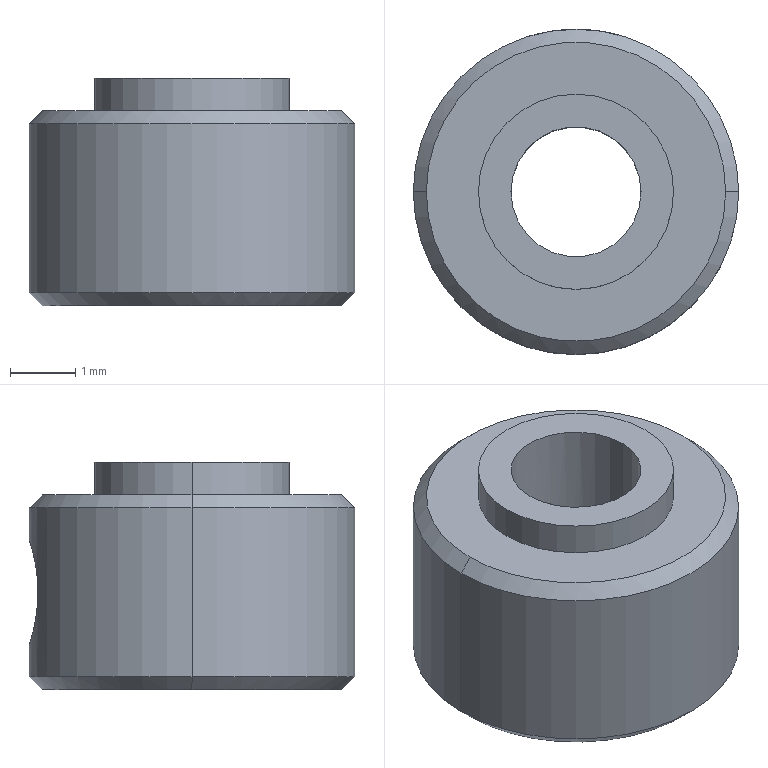Part | SolidWorks | features Chamfer 1, Extrusion 1, HoleWzd 1, ICE 1 | 1 solid | 15 faces | box 5 x 5 x 3.5 mm | volume 47.704 mm3 | cylinder 8 | cone 4 | plane 3 | commonest cylinder face diameters 1.6 x2 2 x2 3 x2 5 x2
STEP:
#1=CARTESIAN_POINT('',(2.3,0.,1.5));
#2=VERTEX_POINT('',#1);
#3=CARTESIAN_POINT('',(-2.3,0.,1.5));
#4=VERTEX_POINT('',#3);
#5=CARTESIAN_POINT('',(0.,0.,1.5));
#6=DIRECTION('',(0.,0.,1.));
#7=DIRECTION('',(1.,0.,0.));
#8=AXIS2_PLACEMENT_3D('',#5,#6,#7);
#9=CIRCLE('',#8,2.3);
#10=EDGE_CURVE('',#2,#4,#9,.T.);
#11=ORIENTED_EDGE('',*,*,#10,.F.);
#12=CARTESIAN_POINT('',(2.5,0.,1.3));
#13=VERTEX_POINT('',#12);
#14=CARTESIAN_POINT('',(2.3,0.,1.5));
#15=DIRECTION('',(0.7071,0.,-0.7071));
#16=VECTOR('',#15,1000.);
#17=LINE('',#14,#16);
#18=EDGE_CURVE('',#2,#13,#17,.T.);
#19=ORIENTED_EDGE('',*,*,#18,.T.);
#20=CARTESIAN_POINT('',(-2.5,0.,1.3));
#21=VERTEX_POINT('',#20);
#22=CARTESIAN_POINT('',(0.,0.,1.3));
#23=DIRECTION('',(0.,0.,-1.));
#24=DIRECTION('',(1.,0.,0.));
#25=AXIS2_PLACEMENT_3D('',#22,#23,#24);
#26=CIRCLE('',#25,2.5);
#27=EDGE_CURVE('',#21,#13,#26,.T.);
#28=ORIENTED_EDGE('',*,*,#27,.F.);
#29=CARTESIAN_POINT('',(-2.3,0.,1.5));
#30=DIRECTION('',(-0.7071,0.,-0.7071));
#31=VECTOR('',#30,1000.);
#32=LINE('',#29,#31);
#33=EDGE_CURVE('',#4,#21,#32,.T.);
#34=ORIENTED_EDGE('',*,*,#33,.F.);
#35=EDGE_LOOP('',(#11,#19,#28,#34));
#36=FACE_OUTER_BOUND('',#35,.T.);
#37=CARTESIAN_POINT('',(0.,0.,1.5));
#38=DIRECTION('',(0.,0.,-1.));
#39=DIRECTION('',(-1.,0.,0.));
#40=AXIS2_PLACEMENT_3D('',#37,#38,#39);
#41=CONICAL_SURFACE('',#40,2.3,0.7854);
#42=ADVANCED_FACE('',(#36),#41,.T.);
#43=CARTESIAN_POINT('',(-2.3,0.,-1.5));
#44=VERTEX_POINT('',#43);
#45=CARTESIAN_POINT('',(2.3,0.,-1.5));
#46=VERTEX_POINT('',#45);
#47=CARTESIAN_POINT('',(0.,0.,-1.5));
#48=DIRECTION('',(0.,0.,-1.));
#49=DIRECTION('',(1.,0.,0.));
#50=AXIS2_PLACEMENT_3D('',#47,#48,#49);
#51=CIRCLE('',#50,2.3);
#52=EDGE_CURVE('',#44,#46,#51,.T.);
#53=ORIENTED_EDGE('',*,*,#52,.F.);
#54=CARTESIAN_POINT('',(-2.5,0.,-1.3));
#55=VERTEX_POINT('',#54);
#56=CARTESIAN_POINT('',(-2.5,0.,-1.3));
#57=DIRECTION('',(-0.7071,0.,0.7071));
#58=VECTOR('',#57,1000.);
#59=LINE('',#56,#58);
#60=EDGE_CURVE('',#44,#55,#59,.T.);
#61=ORIENTED_EDGE('',*,*,#60,.T.);
#62=CARTESIAN_POINT('',(2.5,0.,-1.3));
#63=VERTEX_POINT('',#62);
#64=CARTESIAN_POINT('',(0.,0.,-1.3));
#65=DIRECTION('',(0.,0.,1.));
#66=DIRECTION('',(1.,0.,0.));
#67=AXIS2_PLACEMENT_3D('',#64,#65,#66);
#68=CIRCLE('',#67,2.5);
#69=EDGE_CURVE('',#63,#55,#68,.T.);
#70=ORIENTED_EDGE('',*,*,#69,.F.);
#71=CARTESIAN_POINT('',(2.5,0.,-1.3));
#72=DIRECTION('',(0.7071,0.,0.7071));
#73=VECTOR('',#72,1000.);
#74=LINE('',#71,#73);
#75=EDGE_CURVE('',#46,#63,#74,.T.);
#76=ORIENTED_EDGE('',*,*,#75,.F.);
#77=EDGE_LOOP('',(#53,#61,#70,#76));
#78=FACE_OUTER_BOUND('',#77,.T.);
#79=CARTESIAN_POINT('',(0.,0.,-1.3));
#80=DIRECTION('',(0.,0.,1.));
#81=DIRECTION('',(1.,0.,0.));
#82=AXIS2_PLACEMENT_3D('',#79,#80,#81);
#83=CONICAL_SURFACE('',#82,2.5,0.7854);
#84=ADVANCED_FACE('',(#78),#83,.T.);
#85=CARTESIAN_POINT('',(0.,2.5,0.8));
#86=VERTEX_POINT('',#85);
#87=CARTESIAN_POINT('',(0.,2.5,-0.8));
#88=VERTEX_POINT('',#87);
#89=CARTESIAN_POINT('',(0.,2.5,0.8));
#90=CARTESIAN_POINT('',(-0.1049,2.5,0.8));
#91=CARTESIAN_POINT('',(-0.2107,2.493,0.7788));
#92=CARTESIAN_POINT('',(-0.4037,2.469,0.6985));
#93=CARTESIAN_POINT('',(-0.4919,2.452,0.6395));
#94=CARTESIAN_POINT('',(-0.6396,2.418,0.4918));
#95=CARTESIAN_POINT('',(-0.6982,2.401,0.4046));
#96=CARTESIAN_POINT('',(-0.7791,2.376,0.2099));
#97=CARTESIAN_POINT('',(-0.8,2.369,0.1054));
#98=CARTESIAN_POINT('',(-0.8,2.369,-0.1055));
#99=CARTESIAN_POINT('',(-0.7787,2.376,-0.211));
#100=CARTESIAN_POINT('',(-0.6986,2.401,-0.4036));
#101=CARTESIAN_POINT('',(-0.6391,2.418,-0.4922));
#102=CARTESIAN_POINT('',(-0.4925,2.452,-0.6389));
#103=CARTESIAN_POINT('',(-0.4043,2.469,-0.6982));
#104=CARTESIAN_POINT('',(-0.2111,2.493,-0.7787));
#105=CARTESIAN_POINT('',(-0.1064,2.5,-0.8));
#106=CARTESIAN_POINT('',(0.,2.5,-0.8));
#107=B_SPLINE_CURVE_WITH_KNOTS('',3,(#89,#90,#91,#92,#93,#94,#95,#96,#97,#98,#99,#100,#101,#102,#103,#104,#105,#106),.UNSPECIFIED.,.F.,.F.,(4,2,2,2,2,2,2,2,4),(0.002518,0.002832,0.003147,0.003462,0.003776,0.004091,0.004406,0.00472,0.005035),.UNSPECIFIED.);
#108=EDGE_CURVE('',#86,#88,#107,.T.);
#109=ORIENTED_EDGE('',*,*,#108,.F.);
#110=CARTESIAN_POINT('',(0.,1.,0.8));
#111=VERTEX_POINT('',#110);
#112=CARTESIAN_POINT('',(0.,0.,0.8));
#113=DIRECTION('',(0.,-1.,0.));
#114=VECTOR('',#113,1000.);
#115=LINE('',#112,#114);
#116=EDGE_CURVE('',#86,#111,#115,.T.);
#117=ORIENTED_EDGE('',*,*,#116,.T.);
#118=CARTESIAN_POINT('',(0.,1.,-0.8));
#119=VERTEX_POINT('',#118);
#120=CARTESIAN_POINT('',(0.,1.,0.8));
#121=CARTESIAN_POINT('',(-0.1101,1.,0.8));
#122=CARTESIAN_POINT('',(-0.2209,0.9807,0.7762));
#123=CARTESIAN_POINT('',(-0.4161,0.9151,0.6915));
#124=CARTESIAN_POINT('',(-0.5007,0.8698,0.6318));
#125=CARTESIAN_POINT('',(-0.6401,0.7729,0.49));
#126=CARTESIAN_POINT('',(-0.6961,0.7204,0.4071));
#127=CARTESIAN_POINT('',(-0.7755,0.6341,0.2211));
#128=CARTESIAN_POINT('',(-0.7999,0.6001,0.1121));
#129=CARTESIAN_POINT('',(-0.8001,0.5999,-0.1109));
#130=CARTESIAN_POINT('',(-0.7764,0.6331,-0.2186));
#131=CARTESIAN_POINT('',(-0.6962,0.7203,-0.4072));
#132=CARTESIAN_POINT('',(-0.641,0.7723,-0.489));
#133=CARTESIAN_POINT('',(-0.5007,0.8698,-0.6319));
#134=CARTESIAN_POINT('',(-0.4177,0.9144,-0.6906));
#135=CARTESIAN_POINT('',(-0.2225,0.9804,-0.7758));
#136=CARTESIAN_POINT('',(-0.1119,1.,-0.8));
#137=CARTESIAN_POINT('',(0.,1.,-0.8));
#138=B_SPLINE_CURVE_WITH_KNOTS('',3,(#120,#121,#122,#123,#124,#125,#126,#127,#128,#129,#130,#131,#132,#133,#134,#135,#136,#137),.UNSPECIFIED.,.F.,.F.,(4,2,2,2,2,2,2,2,4),(0.002649,0.002979,0.003309,0.003639,0.003969,0.004299,0.00463,0.00496,0.00529),.UNSPECIFIED.);
#139=EDGE_CURVE('',#111,#119,#138,.T.);
#140=ORIENTED_EDGE('',*,*,#139,.T.);
#141=CARTESIAN_POINT('',(0.,0.,-0.8));
#142=DIRECTION('',(0.,-1.,0.));
#143=VECTOR('',#142,1000.);
#144=LINE('',#141,#143);
#145=EDGE_CURVE('',#88,#119,#144,.T.);
#146=ORIENTED_EDGE('',*,*,#145,.F.);
#147=EDGE_LOOP('',(#109,#117,#140,#146));
#148=FACE_OUTER_BOUND('',#147,.T.);
#149=CARTESIAN_POINT('',(0.,0.,0.));
#150=DIRECTION('',(0.,-1.,0.));
#151=DIRECTION('',(0.,0.,-1.));
#152=AXIS2_PLACEMENT_3D('',#149,#150,#151);
#153=CYLINDRICAL_SURFACE('',#152,0.8);
#154=ADVANCED_FACE('',(#148),#153,.F.);
#155=CARTESIAN_POINT('',(1.5,0.,2.));
#156=VERTEX_POINT('',#155);
#157=CARTESIAN_POINT('',(-1.5,0.,2.));
#158=VERTEX_POINT('',#157);
#159=CARTESIAN_POINT('',(0.,0.,2.));
#160=DIRECTION('',(0.,0.,1.));
#161=DIRECTION('',(1.,0.,0.));
#162=AXIS2_PLACEMENT_3D('',#159,#160,#161);
#163=CIRCLE('',#162,1.5);
#164=EDGE_CURVE('',#156,#158,#163,.T.);
#165=ORIENTED_EDGE('',*,*,#164,.F.);
#166=CARTESIAN_POINT('',(1.5,0.,1.5));
#167=VERTEX_POINT('',#166);
#168=CARTESIAN_POINT('',(1.5,0.,2.));
#169=DIRECTION('',(0.,0.,-1.));
#170=VECTOR('',#169,1000.);
#171=LINE('',#168,#170);
#172=EDGE_CURVE('',#156,#167,#171,.T.);
#173=ORIENTED_EDGE('',*,*,#172,.T.);
#174=CARTESIAN_POINT('',(-1.5,0.,1.5));
#175=VERTEX_POINT('',#174);
#176=CARTESIAN_POINT('',(0.,0.,1.5));
#177=DIRECTION('',(0.,0.,1.));
#178=DIRECTION('',(1.,0.,0.));
#179=AXIS2_PLACEMENT_3D('',#176,#177,#178);
#180=CIRCLE('',#179,1.5);
#181=EDGE_CURVE('',#167,#175,#180,.T.);
#182=ORIENTED_EDGE('',*,*,#181,.T.);
#183=CARTESIAN_POINT('',(-1.5,0.,2.));
#184=DIRECTION('',(0.,0.,-1.));
#185=VECTOR('',#184,1000.);
#186=LINE('',#183,#185);
#187=EDGE_CURVE('',#158,#175,#186,.T.);
#188=ORIENTED_EDGE('',*,*,#187,.F.);
#189=EDGE_LOOP('',(#165,#173,#182,#188));
#190=FACE_OUTER_BOUND('',#189,.T.);
#191=CARTESIAN_POINT('',(0.,0.,2.));
#192=DIRECTION('',(0.,0.,-1.));
#193=DIRECTION('',(-1.,0.,0.));
#194=AXIS2_PLACEMENT_3D('',#191,#192,#193);
#195=CYLINDRICAL_SURFACE('',#194,1.5);
#196=ADVANCED_FACE('',(#190),#195,.T.);
#197=CARTESIAN_POINT('',(-1.,0.,2.));
#198=VERTEX_POINT('',#197);
#199=CARTESIAN_POINT('',(1.,0.,2.));
#200=VERTEX_POINT('',#199);
#201=CARTESIAN_POINT('',(0.,0.,2.));
#202=DIRECTION('',(0.,0.,1.));
#203=DIRECTION('',(1.,0.,0.));
#204=AXIS2_PLACEMENT_3D('',#201,#202,#203);
#205=CIRCLE('',#204,1.);
#206=EDGE_CURVE('',#198,#200,#205,.T.);
#207=ORIENTED_EDGE('',*,*,#206,.T.);
#208=CARTESIAN_POINT('',(1.,0.,-1.5));
#209=VERTEX_POINT('',#208);
#210=CARTESIAN_POINT('',(1.,0.,1.5));
#211=DIRECTION('',(0.,0.,-1.));
#212=VECTOR('',#211,1000.);
#213=LINE('',#210,#212);
#214=EDGE_CURVE('',#200,#209,#213,.T.);
#215=ORIENTED_EDGE('',*,*,#214,.T.);
#216=CARTESIAN_POINT('',(-1.,0.,-1.5));
#217=VERTEX_POINT('',#216);
#218=CARTESIAN_POINT('',(0.,0.,-1.5));
#219=DIRECTION('',(0.,0.,1.));
#220=DIRECTION('',(1.,0.,0.));
#221=AXIS2_PLACEMENT_3D('',#218,#219,#220);
#222=CIRCLE('',#221,1.);
#223=EDGE_CURVE('',#217,#209,#222,.T.);
#224=ORIENTED_EDGE('',*,*,#223,.F.);
#225=CARTESIAN_POINT('',(-1.,0.,1.5));
#226=DIRECTION('',(0.,0.,-1.));
#227=VECTOR('',#226,1000.);
#228=LINE('',#225,#227);
#229=EDGE_CURVE('',#198,#217,#228,.T.);
#230=ORIENTED_EDGE('',*,*,#229,.F.);
#231=EDGE_LOOP('',(#207,#215,#224,#230));
#232=FACE_OUTER_BOUND('',#231,.T.);
#233=CARTESIAN_POINT('',(0.,0.,1.5));
#234=DIRECTION('',(0.,0.,-1.));
#235=DIRECTION('',(-1.,0.,0.));
#236=AXIS2_PLACEMENT_3D('',#233,#234,#235);
#237=CYLINDRICAL_SURFACE('',#236,1.);
#238=ADVANCED_FACE('',(#232),#237,.F.);
#239=CARTESIAN_POINT('',(0.,2.5,-0.8));
#240=CARTESIAN_POINT('',(0.1065,2.5,-0.8));
#241=CARTESIAN_POINT('',(0.2109,2.493,-0.7788));
#242=CARTESIAN_POINT('',(0.4044,2.469,-0.6982));
#243=CARTESIAN_POINT('',(0.4927,2.452,-0.6388));
#244=CARTESIAN_POINT('',(0.6392,2.418,-0.4921));
#245=CARTESIAN_POINT('',(0.6986,2.401,-0.4035));
#246=CARTESIAN_POINT('',(0.7786,2.376,-0.2113));
#247=CARTESIAN_POINT('',(0.7999,2.369,-0.1055));
#248=CARTESIAN_POINT('',(0.8001,2.369,0.1048));
#249=CARTESIAN_POINT('',(0.7791,2.376,0.2099));
#250=CARTESIAN_POINT('',(0.6982,2.401,0.4045));
#251=CARTESIAN_POINT('',(0.6392,2.418,0.4922));
#252=CARTESIAN_POINT('',(0.4917,2.452,0.6396));
#253=CARTESIAN_POINT('',(0.4035,2.469,0.6986));
#254=CARTESIAN_POINT('',(0.2107,2.493,0.7788));
#255=CARTESIAN_POINT('',(0.1049,2.5,0.8));
#256=CARTESIAN_POINT('',(0.,2.5,0.8));
#257=B_SPLINE_CURVE_WITH_KNOTS('',3,(#239,#240,#241,#242,#243,#244,#245,#246,#247,#248,#249,#250,#251,#252,#253,#254,#255,#256),.UNSPECIFIED.,.F.,.F.,(4,2,2,2,2,2,2,2,4),(0.,0.0003147,0.0006295,0.0009442,0.001259,0.001574,0.001888,0.002203,0.002518),.UNSPECIFIED.);
#258=EDGE_CURVE('',#88,#86,#257,.T.);
#259=ORIENTED_EDGE('',*,*,#258,.T.);
#260=ORIENTED_EDGE('',*,*,#108,.T.);
#261=EDGE_LOOP('',(#259,#260));
#262=FACE_BOUND('',#261,.T.);
#263=ORIENTED_EDGE('',*,*,#27,.T.);
#264=CARTESIAN_POINT('',(2.5,0.,1.5));
#265=DIRECTION('',(0.,0.,-1.));
#266=VECTOR('',#265,1000.);
#267=LINE('',#264,#266);
#268=EDGE_CURVE('',#13,#63,#267,.T.);
#269=ORIENTED_EDGE('',*,*,#268,.T.);
#270=ORIENTED_EDGE('',*,*,#69,.T.);
#271=CARTESIAN_POINT('',(-2.5,0.,1.5));
#272=DIRECTION('',(0.,0.,-1.));
#273=VECTOR('',#272,1000.);
#274=LINE('',#271,#273);
#275=EDGE_CURVE('',#21,#55,#274,.T.);
#276=ORIENTED_EDGE('',*,*,#275,.F.);
#277=EDGE_LOOP('',(#263,#269,#270,#276));
#278=FACE_OUTER_BOUND('',#277,.T.);
#279=CARTESIAN_POINT('',(0.,0.,1.5));
#280=DIRECTION('',(0.,0.,-1.));
#281=DIRECTION('',(-1.,0.,0.));
#282=AXIS2_PLACEMENT_3D('',#279,#280,#281);
#283=CYLINDRICAL_SURFACE('',#282,2.5);
#284=ADVANCED_FACE('',(#262,#278),#283,.T.);
#285=CARTESIAN_POINT('',(0.,0.,1.5));
#286=DIRECTION('',(0.,0.,1.));
#287=DIRECTION('',(1.,0.,0.));
#288=AXIS2_PLACEMENT_3D('',#285,#286,#287);
#289=CIRCLE('',#288,2.3);
#290=EDGE_CURVE('',#4,#2,#289,.T.);
#291=ORIENTED_EDGE('',*,*,#290,.T.);
#292=ORIENTED_EDGE('',*,*,#10,.T.);
#293=EDGE_LOOP('',(#291,#292));
#294=FACE_OUTER_BOUND('',#293,.T.);
#295=CARTESIAN_POINT('',(0.,0.,1.5));
#296=DIRECTION('',(0.,0.,1.));
#297=DIRECTION('',(1.,0.,0.));
#298=AXIS2_PLACEMENT_3D('',#295,#296,#297);
#299=CIRCLE('',#298,1.5);
#300=EDGE_CURVE('',#175,#167,#299,.T.);
#301=ORIENTED_EDGE('',*,*,#300,.F.);
#302=ORIENTED_EDGE('',*,*,#181,.F.);
#303=EDGE_LOOP('',(#301,#302));
#304=FACE_BOUND('',#303,.T.);
#305=CARTESIAN_POINT('',(0.,0.,1.5));
#306=DIRECTION('',(0.,0.,1.));
#307=DIRECTION('',(1.,0.,0.));
#308=AXIS2_PLACEMENT_3D('',#305,#306,#307);
#309=PLANE('',#308);
#310=ADVANCED_FACE('',(#294,#304),#309,.T.);
#311=CARTESIAN_POINT('',(0.,0.,-1.5));
#312=DIRECTION('',(0.,0.,-1.));
#313=DIRECTION('',(1.,0.,0.));
#314=AXIS2_PLACEMENT_3D('',#311,#312,#313);
#315=CIRCLE('',#314,2.3);
#316=EDGE_CURVE('',#46,#44,#315,.T.);
#317=ORIENTED_EDGE('',*,*,#316,.T.);
#318=ORIENTED_EDGE('',*,*,#52,.T.);
#319=EDGE_LOOP('',(#317,#318));
#320=FACE_OUTER_BOUND('',#319,.T.);
#321=ORIENTED_EDGE('',*,*,#223,.T.);
#322=CARTESIAN_POINT('',(0.,0.,-1.5));
#323=DIRECTION('',(0.,0.,1.));
#324=DIRECTION('',(1.,0.,0.));
#325=AXIS2_PLACEMENT_3D('',#322,#323,#324);
#326=CIRCLE('',#325,1.);
#327=EDGE_CURVE('',#209,#217,#326,.T.);
#328=ORIENTED_EDGE('',*,*,#327,.T.);
#329=EDGE_LOOP('',(#321,#328));
#330=FACE_BOUND('',#329,.T.);
#331=CARTESIAN_POINT('',(0.,0.,-1.5));
#332=DIRECTION('',(0.,0.,1.));
#333=DIRECTION('',(1.,0.,0.));
#334=AXIS2_PLACEMENT_3D('',#331,#332,#333);
#335=PLANE('',#334);
#336=ADVANCED_FACE('',(#320,#330),#335,.F.);
#337=ORIENTED_EDGE('',*,*,#268,.F.);
#338=CARTESIAN_POINT('',(0.,0.,1.3));
#339=DIRECTION('',(0.,0.,-1.));
#340=DIRECTION('',(1.,0.,0.));
#341=AXIS2_PLACEMENT_3D('',#338,#339,#340);
#342=CIRCLE('',#341,2.5);
#343=EDGE_CURVE('',#13,#21,#342,.T.);
#344=ORIENTED_EDGE('',*,*,#343,.T.);
#345=ORIENTED_EDGE('',*,*,#275,.T.);
#346=CARTESIAN_POINT('',(0.,0.,-1.3));
#347=DIRECTION('',(0.,0.,1.));
#348=DIRECTION('',(1.,0.,0.));
#349=AXIS2_PLACEMENT_3D('',#346,#347,#348);
#350=CIRCLE('',#349,2.5);
#351=EDGE_CURVE('',#55,#63,#350,.T.);
#352=ORIENTED_EDGE('',*,*,#351,.T.);
#353=EDGE_LOOP('',(#337,#344,#345,#352));
#354=FACE_OUTER_BOUND('',#353,.T.);
#355=CARTESIAN_POINT('',(0.,0.,1.5));
#356=DIRECTION('',(0.,0.,-1.));
#357=DIRECTION('',(-1.,0.,0.));
#358=AXIS2_PLACEMENT_3D('',#355,#356,#357);
#359=CYLINDRICAL_SURFACE('',#358,2.5);
#360=ADVANCED_FACE('',(#354),#359,.T.);
#361=ORIENTED_EDGE('',*,*,#214,.F.);
#362=CARTESIAN_POINT('',(0.,0.,2.));
#363=DIRECTION('',(0.,0.,1.));
#364=DIRECTION('',(1.,0.,0.));
#365=AXIS2_PLACEMENT_3D('',#362,#363,#364);
#366=CIRCLE('',#365,1.);
#367=EDGE_CURVE('',#200,#198,#366,.T.);
#368=ORIENTED_EDGE('',*,*,#367,.T.);
#369=ORIENTED_EDGE('',*,*,#229,.T.);
#370=ORIENTED_EDGE('',*,*,#327,.F.);
#371=EDGE_LOOP('',(#361,#368,#369,#370));
#372=FACE_OUTER_BOUND('',#371,.T.);
#373=CARTESIAN_POINT('',(0.,1.,-0.8));
#374=CARTESIAN_POINT('',(0.1122,1.,-0.8));
#375=CARTESIAN_POINT('',(0.2216,0.9805,-0.7759));
#376=CARTESIAN_POINT('',(0.4157,0.9152,-0.6916));
#377=CARTESIAN_POINT('',(0.5007,0.8697,-0.6318));
#378=CARTESIAN_POINT('',(0.64,0.773,-0.4901));
#379=CARTESIAN_POINT('',(0.696,0.7204,-0.4073));
#380=CARTESIAN_POINT('',(0.7758,0.6338,-0.2203));
#381=CARTESIAN_POINT('',(0.8,0.6,-0.1105));
#382=CARTESIAN_POINT('',(0.8,0.6,0.05557));
#383=CARTESIAN_POINT('',(0.794,0.6081,0.1114));
#384=CARTESIAN_POINT('',(0.772,0.6359,0.2167));
#385=CARTESIAN_POINT('',(0.7561,0.6551,0.2664));
#386=CARTESIAN_POINT('',(0.6956,0.7209,0.4083));
#387=CARTESIAN_POINT('',(0.6404,0.7728,0.4898));
#388=CARTESIAN_POINT('',(0.4999,0.8703,0.6325));
#389=CARTESIAN_POINT('',(0.4164,0.915,0.6914));
#390=CARTESIAN_POINT('',(0.221,0.9807,0.7762));
#391=CARTESIAN_POINT('',(0.1105,1.,0.8));
#392=CARTESIAN_POINT('',(0.,1.,0.8));
#393=B_SPLINE_CURVE_WITH_KNOTS('',3,(#373,#374,#375,#376,#377,#378,#379,#380,#381,#382,#383,#384,#385,#386,#387,#388,#389,#390,#391,#392),.UNSPECIFIED.,.F.,.F.,(4,2,2,2,2,2,2,2,2,4),(0.,0.0003311,0.0006623,0.0009934,0.001325,0.00149,0.001656,0.001987,0.002318,0.002649),.UNSPECIFIED.);
#394=EDGE_CURVE('',#119,#111,#393,.T.);
#395=ORIENTED_EDGE('',*,*,#394,.F.);
#396=ORIENTED_EDGE('',*,*,#139,.F.);
#397=EDGE_LOOP('',(#395,#396));
#398=FACE_BOUND('',#397,.T.);
#399=CARTESIAN_POINT('',(0.,0.,1.5));
#400=DIRECTION('',(0.,0.,-1.));
#401=DIRECTION('',(-1.,0.,0.));
#402=AXIS2_PLACEMENT_3D('',#399,#400,#401);
#403=CYLINDRICAL_SURFACE('',#402,1.);
#404=ADVANCED_FACE('',(#372,#398),#403,.F.);
#405=CARTESIAN_POINT('',(0.,0.,2.));
#406=DIRECTION('',(0.,0.,1.));
#407=DIRECTION('',(1.,0.,0.));
#408=AXIS2_PLACEMENT_3D('',#405,#406,#407);
#409=CIRCLE('',#408,1.5);
#410=EDGE_CURVE('',#158,#156,#409,.T.);
#411=ORIENTED_EDGE('',*,*,#410,.T.);
#412=ORIENTED_EDGE('',*,*,#164,.T.);
#413=EDGE_LOOP('',(#411,#412));
#414=FACE_OUTER_BOUND('',#413,.T.);
#415=ORIENTED_EDGE('',*,*,#206,.F.);
#416=ORIENTED_EDGE('',*,*,#367,.F.);
#417=EDGE_LOOP('',(#415,#416));
#418=FACE_BOUND('',#417,.T.);
#419=CARTESIAN_POINT('',(0.,0.,2.));
#420=DIRECTION('',(0.,0.,1.));
#421=DIRECTION('',(1.,0.,0.));
#422=AXIS2_PLACEMENT_3D('',#419,#420,#421);
#423=PLANE('',#422);
#424=ADVANCED_FACE('',(#414,#418),#423,.T.);
#425=ORIENTED_EDGE('',*,*,#172,.F.);
#426=ORIENTED_EDGE('',*,*,#410,.F.);
#427=ORIENTED_EDGE('',*,*,#187,.T.);
#428=ORIENTED_EDGE('',*,*,#300,.T.);
#429=EDGE_LOOP('',(#425,#426,#427,#428));
#430=FACE_OUTER_BOUND('',#429,.T.);
#431=CARTESIAN_POINT('',(0.,0.,2.));
#432=DIRECTION('',(0.,0.,-1.));
#433=DIRECTION('',(-1.,0.,0.));
#434=AXIS2_PLACEMENT_3D('',#431,#432,#433);
#435=CYLINDRICAL_SURFACE('',#434,1.5);
#436=ADVANCED_FACE('',(#430),#435,.T.);
#437=ORIENTED_EDGE('',*,*,#116,.F.);
#438=ORIENTED_EDGE('',*,*,#258,.F.);
#439=ORIENTED_EDGE('',*,*,#145,.T.);
#440=ORIENTED_EDGE('',*,*,#394,.T.);
#441=EDGE_LOOP('',(#437,#438,#439,#440));
#442=FACE_OUTER_BOUND('',#441,.T.);
#443=CARTESIAN_POINT('',(0.,0.,0.));
#444=DIRECTION('',(0.,-1.,0.));
#445=DIRECTION('',(0.,0.,-1.));
#446=AXIS2_PLACEMENT_3D('',#443,#444,#445);
#447=CYLINDRICAL_SURFACE('',#446,0.8);
#448=ADVANCED_FACE('',(#442),#447,.F.);
#449=ORIENTED_EDGE('',*,*,#60,.F.);
#450=ORIENTED_EDGE('',*,*,#316,.F.);
#451=ORIENTED_EDGE('',*,*,#75,.T.);
#452=ORIENTED_EDGE('',*,*,#351,.F.);
#453=EDGE_LOOP('',(#449,#450,#451,#452));
#454=FACE_OUTER_BOUND('',#453,.T.);
#455=CARTESIAN_POINT('',(0.,0.,-1.3));
#456=DIRECTION('',(0.,0.,1.));
#457=DIRECTION('',(1.,0.,0.));
#458=AXIS2_PLACEMENT_3D('',#455,#456,#457);
#459=CONICAL_SURFACE('',#458,2.5,0.7854);
#460=ADVANCED_FACE('',(#454),#459,.T.);
#461=ORIENTED_EDGE('',*,*,#18,.F.);
#462=ORIENTED_EDGE('',*,*,#290,.F.);
#463=ORIENTED_EDGE('',*,*,#33,.T.);
#464=ORIENTED_EDGE('',*,*,#343,.F.);
#465=EDGE_LOOP('',(#461,#462,#463,#464));
#466=FACE_OUTER_BOUND('',#465,.T.);
#467=CARTESIAN_POINT('',(0.,0.,1.5));
#468=DIRECTION('',(0.,0.,-1.));
#469=DIRECTION('',(-1.,0.,0.));
#470=AXIS2_PLACEMENT_3D('',#467,#468,#469);
#471=CONICAL_SURFACE('',#470,2.3,0.7854);
#472=ADVANCED_FACE('',(#466),#471,.T.);
#473=CLOSED_SHELL('',(#42,#84,#154,#196,#238,#284,#310,#336,#360,#404,#424,#436,#448,#460,#472));
#474=MANIFOLD_SOLID_BREP('',#473);
#475=CARTESIAN_POINT('',(0.,0.,0.));
#476=DIRECTION('',(0.,0.,1.));
#477=DIRECTION('',(1.,0.,0.));
#478=AXIS2_PLACEMENT_3D('',#475,#476,#477);
#479=(LENGTH_UNIT()NAMED_UNIT(*)SI_UNIT(.MILLI.,.METRE.));
#480=UNCERTAINTY_MEASURE_WITH_UNIT(LENGTH_MEASURE(0.00001),#479,'','');
#481=(NAMED_UNIT(*)PLANE_ANGLE_UNIT()SI_UNIT($,.RADIAN.));
#482=(NAMED_UNIT(*)SI_UNIT($,.STERADIAN.)SOLID_ANGLE_UNIT());
#483=(GEOMETRIC_REPRESENTATION_CONTEXT(3)GLOBAL_UNCERTAINTY_ASSIGNED_CONTEXT((#480))GLOBAL_UNIT_ASSIGNED_CONTEXT((#479,#481,#482))REPRESENTATION_CONTEXT('',''));
#484=ADVANCED_BREP_SHAPE_REPRESENTATION('',(#474,#478),#483);